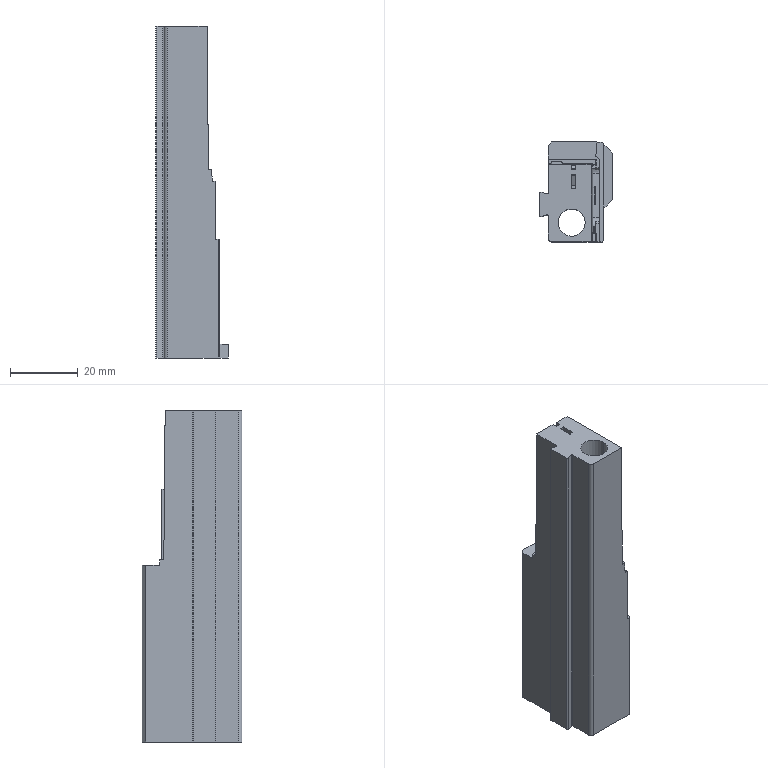Part | Creo | 1 solid | 209 faces | box 21.5 x 29.5 x 98.191 mm | volume 33772 mm3 | plane 111 | other 60 | cylinder 34 | sphere 4 | commonest cylinder face diameters 0.402 x10 0.603 x5 0.6 x4 3.1 x2 3.2 x2 5.166 x2